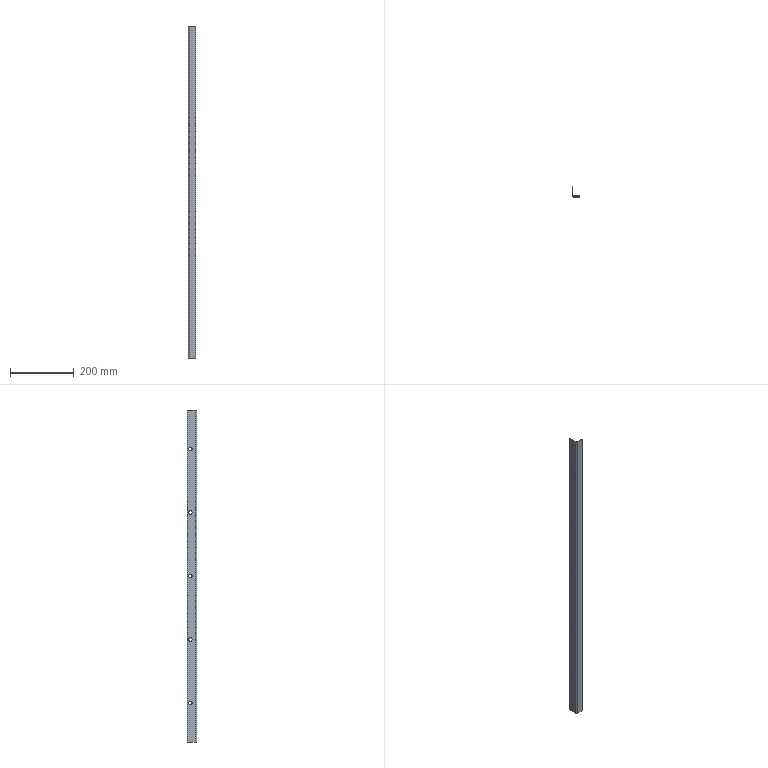Part | STEP file | 750038321 | 1 solid | 20 faces | box 25 x 30 x 1045 mm | volume 131869 mm3 | cylinder 12 | plane 8 | commonest cylinder face diameters 10.5 x10 5 x1 10 x1
STEP:
#1=CARTESIAN_POINT('',(2.5,25.25,200.));
#2=VERTEX_POINT('',#1);
#3=CARTESIAN_POINT('',(2.5,14.75,200.));
#4=VERTEX_POINT('',#3);
#5=CARTESIAN_POINT('',(2.5,20.,200.));
#6=DIRECTION('',(-1.,0.,0.));
#7=DIRECTION('',(0.,-1.,0.));
#8=AXIS2_PLACEMENT_3D('',#5,#6,#7);
#9=CIRCLE('',#8,5.25);
#10=EDGE_CURVE('',#2,#4,#9,.T.);
#11=ORIENTED_EDGE('',*,*,#10,.F.);
#12=CARTESIAN_POINT('',(0.,25.25,200.));
#13=VERTEX_POINT('',#12);
#14=CARTESIAN_POINT('',(1045.729,25.25,200.));
#15=DIRECTION('',(-1.,0.,0.));
#16=VECTOR('',#15,1000.);
#17=LINE('',#14,#16);
#18=EDGE_CURVE('',#2,#13,#17,.T.);
#19=ORIENTED_EDGE('',*,*,#18,.T.);
#20=CARTESIAN_POINT('',(0.,14.75,200.));
#21=VERTEX_POINT('',#20);
#22=CARTESIAN_POINT('',(0.,20.,200.));
#23=DIRECTION('',(1.,0.,0.));
#24=DIRECTION('',(0.,-1.,0.));
#25=AXIS2_PLACEMENT_3D('',#22,#23,#24);
#26=CIRCLE('',#25,5.25);
#27=EDGE_CURVE('',#21,#13,#26,.T.);
#28=ORIENTED_EDGE('',*,*,#27,.F.);
#29=CARTESIAN_POINT('',(1045.729,14.75,200.));
#30=DIRECTION('',(-1.,0.,0.));
#31=VECTOR('',#30,1000.);
#32=LINE('',#29,#31);
#33=EDGE_CURVE('',#4,#21,#32,.T.);
#34=ORIENTED_EDGE('',*,*,#33,.F.);
#35=EDGE_LOOP('',(#11,#19,#28,#34));
#36=FACE_OUTER_BOUND('',#35,.T.);
#37=CARTESIAN_POINT('',(1045.729,20.,200.));
#38=DIRECTION('',(-1.,0.,0.));
#39=DIRECTION('',(0.,-1.,0.));
#40=AXIS2_PLACEMENT_3D('',#37,#38,#39);
#41=CYLINDRICAL_SURFACE('',#40,5.25);
#42=ADVANCED_FACE('',(#36),#41,.F.);
#43=CARTESIAN_POINT('',(2.5,25.25,-200.));
#44=VERTEX_POINT('',#43);
#45=CARTESIAN_POINT('',(2.5,14.75,-200.));
#46=VERTEX_POINT('',#45);
#47=CARTESIAN_POINT('',(2.5,20.,-200.));
#48=DIRECTION('',(-1.,0.,0.));
#49=DIRECTION('',(0.,-1.,0.));
#50=AXIS2_PLACEMENT_3D('',#47,#48,#49);
#51=CIRCLE('',#50,5.25);
#52=EDGE_CURVE('',#44,#46,#51,.T.);
#53=ORIENTED_EDGE('',*,*,#52,.F.);
#54=CARTESIAN_POINT('',(0.,25.25,-200.));
#55=VERTEX_POINT('',#54);
#56=CARTESIAN_POINT('',(1045.729,25.25,-200.));
#57=DIRECTION('',(-1.,0.,0.));
#58=VECTOR('',#57,1000.);
#59=LINE('',#56,#58);
#60=EDGE_CURVE('',#44,#55,#59,.T.);
#61=ORIENTED_EDGE('',*,*,#60,.T.);
#62=CARTESIAN_POINT('',(0.,14.75,-200.));
#63=VERTEX_POINT('',#62);
#64=CARTESIAN_POINT('',(0.,20.,-200.));
#65=DIRECTION('',(1.,0.,0.));
#66=DIRECTION('',(0.,-1.,0.));
#67=AXIS2_PLACEMENT_3D('',#64,#65,#66);
#68=CIRCLE('',#67,5.25);
#69=EDGE_CURVE('',#63,#55,#68,.T.);
#70=ORIENTED_EDGE('',*,*,#69,.F.);
#71=CARTESIAN_POINT('',(1045.729,14.75,-200.));
#72=DIRECTION('',(-1.,0.,0.));
#73=VECTOR('',#72,1000.);
#74=LINE('',#71,#73);
#75=EDGE_CURVE('',#46,#63,#74,.T.);
#76=ORIENTED_EDGE('',*,*,#75,.F.);
#77=EDGE_LOOP('',(#53,#61,#70,#76));
#78=FACE_OUTER_BOUND('',#77,.T.);
#79=CARTESIAN_POINT('',(1045.729,20.,-200.));
#80=DIRECTION('',(-1.,0.,0.));
#81=DIRECTION('',(0.,-1.,0.));
#82=AXIS2_PLACEMENT_3D('',#79,#80,#81);
#83=CYLINDRICAL_SURFACE('',#82,5.25);
#84=ADVANCED_FACE('',(#78),#83,.F.);
#85=CARTESIAN_POINT('',(2.5,25.25,-400.));
#86=VERTEX_POINT('',#85);
#87=CARTESIAN_POINT('',(2.5,14.75,-400.));
#88=VERTEX_POINT('',#87);
#89=CARTESIAN_POINT('',(2.5,20.,-400.));
#90=DIRECTION('',(-1.,0.,0.));
#91=DIRECTION('',(0.,-1.,0.));
#92=AXIS2_PLACEMENT_3D('',#89,#90,#91);
#93=CIRCLE('',#92,5.25);
#94=EDGE_CURVE('',#86,#88,#93,.T.);
#95=ORIENTED_EDGE('',*,*,#94,.F.);
#96=CARTESIAN_POINT('',(0.,25.25,-400.));
#97=VERTEX_POINT('',#96);
#98=CARTESIAN_POINT('',(1045.729,25.25,-400.));
#99=DIRECTION('',(-1.,0.,0.));
#100=VECTOR('',#99,1000.);
#101=LINE('',#98,#100);
#102=EDGE_CURVE('',#86,#97,#101,.T.);
#103=ORIENTED_EDGE('',*,*,#102,.T.);
#104=CARTESIAN_POINT('',(0.,14.75,-400.));
#105=VERTEX_POINT('',#104);
#106=CARTESIAN_POINT('',(0.,20.,-400.));
#107=DIRECTION('',(1.,0.,0.));
#108=DIRECTION('',(0.,-1.,0.));
#109=AXIS2_PLACEMENT_3D('',#106,#107,#108);
#110=CIRCLE('',#109,5.25);
#111=EDGE_CURVE('',#105,#97,#110,.T.);
#112=ORIENTED_EDGE('',*,*,#111,.F.);
#113=CARTESIAN_POINT('',(1045.729,14.75,-400.));
#114=DIRECTION('',(-1.,0.,0.));
#115=VECTOR('',#114,1000.);
#116=LINE('',#113,#115);
#117=EDGE_CURVE('',#88,#105,#116,.T.);
#118=ORIENTED_EDGE('',*,*,#117,.F.);
#119=EDGE_LOOP('',(#95,#103,#112,#118));
#120=FACE_OUTER_BOUND('',#119,.T.);
#121=CARTESIAN_POINT('',(1045.729,20.,-400.));
#122=DIRECTION('',(-1.,0.,0.));
#123=DIRECTION('',(0.,-1.,0.));
#124=AXIS2_PLACEMENT_3D('',#121,#122,#123);
#125=CYLINDRICAL_SURFACE('',#124,5.25);
#126=ADVANCED_FACE('',(#120),#125,.F.);
#127=CARTESIAN_POINT('',(2.5,25.25,0.));
#128=VERTEX_POINT('',#127);
#129=CARTESIAN_POINT('',(2.5,14.75,0.));
#130=VERTEX_POINT('',#129);
#131=CARTESIAN_POINT('',(2.5,20.,0.));
#132=DIRECTION('',(-1.,0.,0.));
#133=DIRECTION('',(0.,-1.,0.));
#134=AXIS2_PLACEMENT_3D('',#131,#132,#133);
#135=CIRCLE('',#134,5.25);
#136=EDGE_CURVE('',#128,#130,#135,.T.);
#137=ORIENTED_EDGE('',*,*,#136,.F.);
#138=CARTESIAN_POINT('',(0.,25.25,0.));
#139=VERTEX_POINT('',#138);
#140=CARTESIAN_POINT('',(1045.729,25.25,0.));
#141=DIRECTION('',(-1.,0.,0.));
#142=VECTOR('',#141,1000.);
#143=LINE('',#140,#142);
#144=EDGE_CURVE('',#128,#139,#143,.T.);
#145=ORIENTED_EDGE('',*,*,#144,.T.);
#146=CARTESIAN_POINT('',(0.,14.75,0.));
#147=VERTEX_POINT('',#146);
#148=CARTESIAN_POINT('',(0.,20.,0.));
#149=DIRECTION('',(1.,0.,0.));
#150=DIRECTION('',(0.,-1.,0.));
#151=AXIS2_PLACEMENT_3D('',#148,#149,#150);
#152=CIRCLE('',#151,5.25);
#153=EDGE_CURVE('',#147,#139,#152,.T.);
#154=ORIENTED_EDGE('',*,*,#153,.F.);
#155=CARTESIAN_POINT('',(1045.729,14.75,0.));
#156=DIRECTION('',(-1.,0.,0.));
#157=VECTOR('',#156,1000.);
#158=LINE('',#155,#157);
#159=EDGE_CURVE('',#130,#147,#158,.T.);
#160=ORIENTED_EDGE('',*,*,#159,.F.);
#161=EDGE_LOOP('',(#137,#145,#154,#160));
#162=FACE_OUTER_BOUND('',#161,.T.);
#163=CARTESIAN_POINT('',(1045.729,20.,0.));
#164=DIRECTION('',(-1.,0.,0.));
#165=DIRECTION('',(0.,-1.,0.));
#166=AXIS2_PLACEMENT_3D('',#163,#164,#165);
#167=CYLINDRICAL_SURFACE('',#166,5.25);
#168=ADVANCED_FACE('',(#162),#167,.F.);
#169=CARTESIAN_POINT('',(2.5,25.25,400.));
#170=VERTEX_POINT('',#169);
#171=CARTESIAN_POINT('',(2.5,14.75,400.));
#172=VERTEX_POINT('',#171);
#173=CARTESIAN_POINT('',(2.5,20.,400.));
#174=DIRECTION('',(-1.,0.,0.));
#175=DIRECTION('',(0.,-1.,0.));
#176=AXIS2_PLACEMENT_3D('',#173,#174,#175);
#177=CIRCLE('',#176,5.25);
#178=EDGE_CURVE('',#170,#172,#177,.T.);
#179=ORIENTED_EDGE('',*,*,#178,.F.);
#180=CARTESIAN_POINT('',(0.,25.25,400.));
#181=VERTEX_POINT('',#180);
#182=CARTESIAN_POINT('',(1045.729,25.25,400.));
#183=DIRECTION('',(-1.,0.,0.));
#184=VECTOR('',#183,1000.);
#185=LINE('',#182,#184);
#186=EDGE_CURVE('',#170,#181,#185,.T.);
#187=ORIENTED_EDGE('',*,*,#186,.T.);
#188=CARTESIAN_POINT('',(0.,14.75,400.));
#189=VERTEX_POINT('',#188);
#190=CARTESIAN_POINT('',(0.,20.,400.));
#191=DIRECTION('',(1.,0.,0.));
#192=DIRECTION('',(0.,-1.,0.));
#193=AXIS2_PLACEMENT_3D('',#190,#191,#192);
#194=CIRCLE('',#193,5.25);
#195=EDGE_CURVE('',#189,#181,#194,.T.);
#196=ORIENTED_EDGE('',*,*,#195,.F.);
#197=CARTESIAN_POINT('',(1045.729,14.75,400.));
#198=DIRECTION('',(-1.,0.,0.));
#199=VECTOR('',#198,1000.);
#200=LINE('',#197,#199);
#201=EDGE_CURVE('',#172,#189,#200,.T.);
#202=ORIENTED_EDGE('',*,*,#201,.F.);
#203=EDGE_LOOP('',(#179,#187,#196,#202));
#204=FACE_OUTER_BOUND('',#203,.T.);
#205=CARTESIAN_POINT('',(1045.729,20.,400.));
#206=DIRECTION('',(-1.,0.,0.));
#207=DIRECTION('',(0.,-1.,0.));
#208=AXIS2_PLACEMENT_3D('',#205,#206,#207);
#209=CYLINDRICAL_SURFACE('',#208,5.25);
#210=ADVANCED_FACE('',(#204),#209,.F.);
#211=CARTESIAN_POINT('',(0.,5.,522.5));
#212=VERTEX_POINT('',#211);
#213=CARTESIAN_POINT('',(0.,30.,522.5));
#214=VERTEX_POINT('',#213);
#215=CARTESIAN_POINT('',(0.,0.,522.5));
#216=DIRECTION('',(0.,1.,0.));
#217=VECTOR('',#216,1000.);
#218=LINE('',#215,#217);
#219=EDGE_CURVE('',#212,#214,#218,.T.);
#220=ORIENTED_EDGE('',*,*,#219,.T.);
#221=CARTESIAN_POINT('',(0.,30.,-522.5));
#222=VERTEX_POINT('',#221);
#223=CARTESIAN_POINT('',(0.,30.,522.5));
#224=DIRECTION('',(0.,0.,-1.));
#225=VECTOR('',#224,1000.);
#226=LINE('',#223,#225);
#227=EDGE_CURVE('',#214,#222,#226,.T.);
#228=ORIENTED_EDGE('',*,*,#227,.T.);
#229=CARTESIAN_POINT('',(0.,5.,-522.5));
#230=VERTEX_POINT('',#229);
#231=CARTESIAN_POINT('',(0.,0.,-522.5));
#232=DIRECTION('',(0.,-1.,0.));
#233=VECTOR('',#232,1000.);
#234=LINE('',#231,#233);
#235=EDGE_CURVE('',#222,#230,#234,.T.);
#236=ORIENTED_EDGE('',*,*,#235,.T.);
#237=CARTESIAN_POINT('',(0.,5.,522.5));
#238=DIRECTION('',(0.,0.,1.));
#239=VECTOR('',#238,1000.);
#240=LINE('',#237,#239);
#241=EDGE_CURVE('',#230,#212,#240,.T.);
#242=ORIENTED_EDGE('',*,*,#241,.T.);
#243=EDGE_LOOP('',(#220,#228,#236,#242));
#244=FACE_OUTER_BOUND('',#243,.T.);
#245=ORIENTED_EDGE('',*,*,#27,.T.);
#246=CARTESIAN_POINT('',(0.,20.,200.));
#247=DIRECTION('',(1.,0.,0.));
#248=DIRECTION('',(0.,-1.,0.));
#249=AXIS2_PLACEMENT_3D('',#246,#247,#248);
#250=CIRCLE('',#249,5.25);
#251=EDGE_CURVE('',#13,#21,#250,.T.);
#252=ORIENTED_EDGE('',*,*,#251,.T.);
#253=EDGE_LOOP('',(#245,#252));
#254=FACE_BOUND('',#253,.T.);
#255=ORIENTED_EDGE('',*,*,#69,.T.);
#256=CARTESIAN_POINT('',(0.,20.,-200.));
#257=DIRECTION('',(1.,0.,0.));
#258=DIRECTION('',(0.,-1.,0.));
#259=AXIS2_PLACEMENT_3D('',#256,#257,#258);
#260=CIRCLE('',#259,5.25);
#261=EDGE_CURVE('',#55,#63,#260,.T.);
#262=ORIENTED_EDGE('',*,*,#261,.T.);
#263=EDGE_LOOP('',(#255,#262));
#264=FACE_BOUND('',#263,.T.);
#265=ORIENTED_EDGE('',*,*,#111,.T.);
#266=CARTESIAN_POINT('',(0.,20.,-400.));
#267=DIRECTION('',(1.,0.,0.));
#268=DIRECTION('',(0.,-1.,0.));
#269=AXIS2_PLACEMENT_3D('',#266,#267,#268);
#270=CIRCLE('',#269,5.25);
#271=EDGE_CURVE('',#97,#105,#270,.T.);
#272=ORIENTED_EDGE('',*,*,#271,.T.);
#273=EDGE_LOOP('',(#265,#272));
#274=FACE_BOUND('',#273,.T.);
#275=ORIENTED_EDGE('',*,*,#153,.T.);
#276=CARTESIAN_POINT('',(0.,20.,0.));
#277=DIRECTION('',(1.,0.,0.));
#278=DIRECTION('',(0.,-1.,0.));
#279=AXIS2_PLACEMENT_3D('',#276,#277,#278);
#280=CIRCLE('',#279,5.25);
#281=EDGE_CURVE('',#139,#147,#280,.T.);
#282=ORIENTED_EDGE('',*,*,#281,.T.);
#283=EDGE_LOOP('',(#275,#282));
#284=FACE_BOUND('',#283,.T.);
#285=ORIENTED_EDGE('',*,*,#195,.T.);
#286=CARTESIAN_POINT('',(0.,20.,400.));
#287=DIRECTION('',(1.,0.,0.));
#288=DIRECTION('',(0.,-1.,0.));
#289=AXIS2_PLACEMENT_3D('',#286,#287,#288);
#290=CIRCLE('',#289,5.25);
#291=EDGE_CURVE('',#181,#189,#290,.T.);
#292=ORIENTED_EDGE('',*,*,#291,.T.);
#293=EDGE_LOOP('',(#285,#292));
#294=FACE_BOUND('',#293,.T.);
#295=CARTESIAN_POINT('',(0.,0.,522.5));
#296=DIRECTION('',(-1.,0.,0.));
#297=DIRECTION('',(0.,-1.,0.));
#298=AXIS2_PLACEMENT_3D('',#295,#296,#297);
#299=PLANE('',#298);
#300=ADVANCED_FACE('',(#244,#254,#264,#274,#284,#294),#299,.T.);
#301=CARTESIAN_POINT('',(2.5,30.,-522.5));
#302=VERTEX_POINT('',#301);
#303=CARTESIAN_POINT('',(0.,30.,-522.5));
#304=DIRECTION('',(-1.,0.,0.));
#305=VECTOR('',#304,1000.);
#306=LINE('',#303,#305);
#307=EDGE_CURVE('',#302,#222,#306,.T.);
#308=ORIENTED_EDGE('',*,*,#307,.T.);
#309=ORIENTED_EDGE('',*,*,#227,.F.);
#310=CARTESIAN_POINT('',(2.5,30.,522.5));
#311=VERTEX_POINT('',#310);
#312=CARTESIAN_POINT('',(0.,30.,522.5));
#313=DIRECTION('',(1.,0.,0.));
#314=VECTOR('',#313,1000.);
#315=LINE('',#312,#314);
#316=EDGE_CURVE('',#214,#311,#315,.T.);
#317=ORIENTED_EDGE('',*,*,#316,.T.);
#318=CARTESIAN_POINT('',(2.5,30.,522.5));
#319=DIRECTION('',(0.,0.,-1.));
#320=VECTOR('',#319,1000.);
#321=LINE('',#318,#320);
#322=EDGE_CURVE('',#311,#302,#321,.T.);
#323=ORIENTED_EDGE('',*,*,#322,.T.);
#324=EDGE_LOOP('',(#308,#309,#317,#323));
#325=FACE_OUTER_BOUND('',#324,.T.);
#326=CARTESIAN_POINT('',(0.,30.,522.5));
#327=DIRECTION('',(0.,1.,0.));
#328=DIRECTION('',(-1.,0.,0.));
#329=AXIS2_PLACEMENT_3D('',#326,#327,#328);
#330=PLANE('',#329);
#331=ADVANCED_FACE('',(#325),#330,.T.);
#332=CARTESIAN_POINT('',(2.5,5.,522.5));
#333=VERTEX_POINT('',#332);
#334=CARTESIAN_POINT('',(2.5,0.,522.5));
#335=DIRECTION('',(0.,1.,0.));
#336=VECTOR('',#335,1000.);
#337=LINE('',#334,#336);
#338=EDGE_CURVE('',#333,#311,#337,.T.);
#339=ORIENTED_EDGE('',*,*,#338,.T.);
#340=ORIENTED_EDGE('',*,*,#316,.F.);
#341=ORIENTED_EDGE('',*,*,#219,.F.);
#342=CARTESIAN_POINT('',(5.,0.,522.5));
#343=VERTEX_POINT('',#342);
#344=CARTESIAN_POINT('',(5.,5.,522.5));
#345=DIRECTION('',(0.,0.,1.));
#346=DIRECTION('',(-1.,0.,0.));
#347=AXIS2_PLACEMENT_3D('',#344,#345,#346);
#348=CIRCLE('',#347,5.);
#349=EDGE_CURVE('',#212,#343,#348,.T.);
#350=ORIENTED_EDGE('',*,*,#349,.T.);
#351=CARTESIAN_POINT('',(25.,0.,522.5));
#352=VERTEX_POINT('',#351);
#353=CARTESIAN_POINT('',(0.,0.,522.5));
#354=DIRECTION('',(1.,0.,0.));
#355=VECTOR('',#354,1000.);
#356=LINE('',#353,#355);
#357=EDGE_CURVE('',#343,#352,#356,.T.);
#358=ORIENTED_EDGE('',*,*,#357,.T.);
#359=CARTESIAN_POINT('',(25.,2.5,522.5));
#360=VERTEX_POINT('',#359);
#361=CARTESIAN_POINT('',(25.,0.,522.5));
#362=DIRECTION('',(0.,1.,0.));
#363=VECTOR('',#362,1000.);
#364=LINE('',#361,#363);
#365=EDGE_CURVE('',#352,#360,#364,.T.);
#366=ORIENTED_EDGE('',*,*,#365,.T.);
#367=CARTESIAN_POINT('',(5.,2.5,522.5));
#368=VERTEX_POINT('',#367);
#369=CARTESIAN_POINT('',(0.,2.5,522.5));
#370=DIRECTION('',(-1.,0.,0.));
#371=VECTOR('',#370,1000.);
#372=LINE('',#369,#371);
#373=EDGE_CURVE('',#360,#368,#372,.T.);
#374=ORIENTED_EDGE('',*,*,#373,.T.);
#375=CARTESIAN_POINT('',(5.,5.,522.5));
#376=DIRECTION('',(0.,0.,-1.));
#377=DIRECTION('',(-1.,0.,0.));
#378=AXIS2_PLACEMENT_3D('',#375,#376,#377);
#379=CIRCLE('',#378,2.5);
#380=EDGE_CURVE('',#368,#333,#379,.T.);
#381=ORIENTED_EDGE('',*,*,#380,.T.);
#382=EDGE_LOOP('',(#339,#340,#341,#350,#358,#366,#374,#381));
#383=FACE_OUTER_BOUND('',#382,.T.);
#384=CARTESIAN_POINT('',(0.,0.,522.5));
#385=DIRECTION('',(0.,0.,1.));
#386=DIRECTION('',(1.,0.,0.));
#387=AXIS2_PLACEMENT_3D('',#384,#385,#386);
#388=PLANE('',#387);
#389=ADVANCED_FACE('',(#383),#388,.T.);
#390=ORIENTED_EDGE('',*,*,#349,.F.);
#391=ORIENTED_EDGE('',*,*,#241,.F.);
#392=CARTESIAN_POINT('',(5.,0.,-522.5));
#393=VERTEX_POINT('',#392);
#394=CARTESIAN_POINT('',(5.,5.,-522.5));
#395=DIRECTION('',(0.,0.,1.));
#396=DIRECTION('',(-1.,0.,0.));
#397=AXIS2_PLACEMENT_3D('',#394,#395,#396);
#398=CIRCLE('',#397,5.);
#399=EDGE_CURVE('',#230,#393,#398,.T.);
#400=ORIENTED_EDGE('',*,*,#399,.T.);
#401=CARTESIAN_POINT('',(5.,0.,522.5));
#402=DIRECTION('',(0.,0.,1.));
#403=VECTOR('',#402,1000.);
#404=LINE('',#401,#403);
#405=EDGE_CURVE('',#393,#343,#404,.T.);
#406=ORIENTED_EDGE('',*,*,#405,.T.);
#407=EDGE_LOOP('',(#390,#391,#400,#406));
#408=FACE_OUTER_BOUND('',#407,.T.);
#409=CARTESIAN_POINT('',(5.,5.,522.5));
#410=DIRECTION('',(0.,0.,-1.));
#411=DIRECTION('',(-1.,0.,0.));
#412=AXIS2_PLACEMENT_3D('',#409,#410,#411);
#413=CYLINDRICAL_SURFACE('',#412,5.);
#414=ADVANCED_FACE('',(#408),#413,.T.);
#415=ORIENTED_EDGE('',*,*,#399,.F.);
#416=ORIENTED_EDGE('',*,*,#235,.F.);
#417=ORIENTED_EDGE('',*,*,#307,.F.);
#418=CARTESIAN_POINT('',(2.5,5.,-522.5));
#419=VERTEX_POINT('',#418);
#420=CARTESIAN_POINT('',(2.5,0.,-522.5));
#421=DIRECTION('',(0.,1.,0.));
#422=VECTOR('',#421,1000.);
#423=LINE('',#420,#422);
#424=EDGE_CURVE('',#419,#302,#423,.T.);
#425=ORIENTED_EDGE('',*,*,#424,.F.);
#426=CARTESIAN_POINT('',(5.,2.5,-522.5));
#427=VERTEX_POINT('',#426);
#428=CARTESIAN_POINT('',(5.,5.,-522.5));
#429=DIRECTION('',(0.,0.,-1.));
#430=DIRECTION('',(-1.,0.,0.));
#431=AXIS2_PLACEMENT_3D('',#428,#429,#430);
#432=CIRCLE('',#431,2.5);
#433=EDGE_CURVE('',#427,#419,#432,.T.);
#434=ORIENTED_EDGE('',*,*,#433,.F.);
#435=CARTESIAN_POINT('',(25.,2.5,-522.5));
#436=VERTEX_POINT('',#435);
#437=CARTESIAN_POINT('',(25.,2.5,-522.5));
#438=DIRECTION('',(-1.,0.,0.));
#439=VECTOR('',#438,1000.);
#440=LINE('',#437,#439);
#441=EDGE_CURVE('',#436,#427,#440,.T.);
#442=ORIENTED_EDGE('',*,*,#441,.F.);
#443=CARTESIAN_POINT('',(25.,0.,-522.5));
#444=VERTEX_POINT('',#443);
#445=CARTESIAN_POINT('',(25.,0.,-522.5));
#446=DIRECTION('',(0.,1.,0.));
#447=VECTOR('',#446,1000.);
#448=LINE('',#445,#447);
#449=EDGE_CURVE('',#444,#436,#448,.T.);
#450=ORIENTED_EDGE('',*,*,#449,.F.);
#451=CARTESIAN_POINT('',(25.,0.,-522.5));
#452=DIRECTION('',(1.,0.,0.));
#453=VECTOR('',#452,1000.);
#454=LINE('',#451,#453);
#455=EDGE_CURVE('',#393,#444,#454,.T.);
#456=ORIENTED_EDGE('',*,*,#455,.F.);
#457=EDGE_LOOP('',(#415,#416,#417,#425,#434,#442,#450,#456));
#458=FACE_OUTER_BOUND('',#457,.T.);
#459=CARTESIAN_POINT('',(25.,0.,-522.5));
#460=DIRECTION('',(0.,0.,1.));
#461=DIRECTION('',(1.,0.,0.));
#462=AXIS2_PLACEMENT_3D('',#459,#460,#461);
#463=PLANE('',#462);
#464=ADVANCED_FACE('',(#458),#463,.F.);
#465=ORIENTED_EDGE('',*,*,#18,.F.);
#466=CARTESIAN_POINT('',(2.5,20.,200.));
#467=DIRECTION('',(-1.,0.,0.));
#468=DIRECTION('',(0.,-1.,0.));
#469=AXIS2_PLACEMENT_3D('',#466,#467,#468);
#470=CIRCLE('',#469,5.25);
#471=EDGE_CURVE('',#4,#2,#470,.T.);
#472=ORIENTED_EDGE('',*,*,#471,.F.);
#473=ORIENTED_EDGE('',*,*,#33,.T.);
#474=ORIENTED_EDGE('',*,*,#251,.F.);
#475=EDGE_LOOP('',(#465,#472,#473,#474));
#476=FACE_OUTER_BOUND('',#475,.T.);
#477=CARTESIAN_POINT('',(1045.729,20.,200.));
#478=DIRECTION('',(-1.,0.,0.));
#479=DIRECTION('',(0.,-1.,0.));
#480=AXIS2_PLACEMENT_3D('',#477,#478,#479);
#481=CYLINDRICAL_SURFACE('',#480,5.25);
#482=ADVANCED_FACE('',(#476),#481,.F.);
#483=ORIENTED_EDGE('',*,*,#60,.F.);
#484=CARTESIAN_POINT('',(2.5,20.,-200.));
#485=DIRECTION('',(-1.,0.,0.));
#486=DIRECTION('',(0.,-1.,0.));
#487=AXIS2_PLACEMENT_3D('',#484,#485,#486);
#488=CIRCLE('',#487,5.25);
#489=EDGE_CURVE('',#46,#44,#488,.T.);
#490=ORIENTED_EDGE('',*,*,#489,.F.);
#491=ORIENTED_EDGE('',*,*,#75,.T.);
#492=ORIENTED_EDGE('',*,*,#261,.F.);
#493=EDGE_LOOP('',(#483,#490,#491,#492));
#494=FACE_OUTER_BOUND('',#493,.T.);
#495=CARTESIAN_POINT('',(1045.729,20.,-200.));
#496=DIRECTION('',(-1.,0.,0.));
#497=DIRECTION('',(0.,-1.,0.));
#498=AXIS2_PLACEMENT_3D('',#495,#496,#497);
#499=CYLINDRICAL_SURFACE('',#498,5.25);
#500=ADVANCED_FACE('',(#494),#499,.F.);
#501=ORIENTED_EDGE('',*,*,#102,.F.);
#502=CARTESIAN_POINT('',(2.5,20.,-400.));
#503=DIRECTION('',(-1.,0.,0.));
#504=DIRECTION('',(0.,-1.,0.));
#505=AXIS2_PLACEMENT_3D('',#502,#503,#504);
#506=CIRCLE('',#505,5.25);
#507=EDGE_CURVE('',#88,#86,#506,.T.);
#508=ORIENTED_EDGE('',*,*,#507,.F.);
#509=ORIENTED_EDGE('',*,*,#117,.T.);
#510=ORIENTED_EDGE('',*,*,#271,.F.);
#511=EDGE_LOOP('',(#501,#508,#509,#510));
#512=FACE_OUTER_BOUND('',#511,.T.);
#513=CARTESIAN_POINT('',(1045.729,20.,-400.));
#514=DIRECTION('',(-1.,0.,0.));
#515=DIRECTION('',(0.,-1.,0.));
#516=AXIS2_PLACEMENT_3D('',#513,#514,#515);
#517=CYLINDRICAL_SURFACE('',#516,5.25);
#518=ADVANCED_FACE('',(#512),#517,.F.);
#519=ORIENTED_EDGE('',*,*,#144,.F.);
#520=CARTESIAN_POINT('',(2.5,20.,0.));
#521=DIRECTION('',(-1.,0.,0.));
#522=DIRECTION('',(0.,-1.,0.));
#523=AXIS2_PLACEMENT_3D('',#520,#521,#522);
#524=CIRCLE('',#523,5.25);
#525=EDGE_CURVE('',#130,#128,#524,.T.);
#526=ORIENTED_EDGE('',*,*,#525,.F.);
#527=ORIENTED_EDGE('',*,*,#159,.T.);
#528=ORIENTED_EDGE('',*,*,#281,.F.);
#529=EDGE_LOOP('',(#519,#526,#527,#528));
#530=FACE_OUTER_BOUND('',#529,.T.);
#531=CARTESIAN_POINT('',(1045.729,20.,0.));
#532=DIRECTION('',(-1.,0.,0.));
#533=DIRECTION('',(0.,-1.,0.));
#534=AXIS2_PLACEMENT_3D('',#531,#532,#533);
#535=CYLINDRICAL_SURFACE('',#534,5.25);
#536=ADVANCED_FACE('',(#530),#535,.F.);
#537=ORIENTED_EDGE('',*,*,#186,.F.);
#538=CARTESIAN_POINT('',(2.5,20.,400.));
#539=DIRECTION('',(-1.,0.,0.));
#540=DIRECTION('',(0.,-1.,0.));
#541=AXIS2_PLACEMENT_3D('',#538,#539,#540);
#542=CIRCLE('',#541,5.25);
#543=EDGE_CURVE('',#172,#170,#542,.T.);
#544=ORIENTED_EDGE('',*,*,#543,.F.);
#545=ORIENTED_EDGE('',*,*,#201,.T.);
#546=ORIENTED_EDGE('',*,*,#291,.F.);
#547=EDGE_LOOP('',(#537,#544,#545,#546));
#548=FACE_OUTER_BOUND('',#547,.T.);
#549=CARTESIAN_POINT('',(1045.729,20.,400.));
#550=DIRECTION('',(-1.,0.,0.));
#551=DIRECTION('',(0.,-1.,0.));
#552=AXIS2_PLACEMENT_3D('',#549,#550,#551);
#553=CYLINDRICAL_SURFACE('',#552,5.25);
#554=ADVANCED_FACE('',(#548),#553,.F.);
#555=ORIENTED_EDGE('',*,*,#322,.F.);
#556=ORIENTED_EDGE('',*,*,#338,.F.);
#557=CARTESIAN_POINT('',(2.5,5.,522.5));
#558=DIRECTION('',(0.,0.,1.));
#559=VECTOR('',#558,1000.);
#560=LINE('',#557,#559);
#561=EDGE_CURVE('',#419,#333,#560,.T.);
#562=ORIENTED_EDGE('',*,*,#561,.F.);
#563=ORIENTED_EDGE('',*,*,#424,.T.);
#564=EDGE_LOOP('',(#555,#556,#562,#563));
#565=FACE_OUTER_BOUND('',#564,.T.);
#566=ORIENTED_EDGE('',*,*,#471,.T.);
#567=ORIENTED_EDGE('',*,*,#10,.T.);
#568=EDGE_LOOP('',(#566,#567));
#569=FACE_BOUND('',#568,.T.);
#570=ORIENTED_EDGE('',*,*,#489,.T.);
#571=ORIENTED_EDGE('',*,*,#52,.T.);
#572=EDGE_LOOP('',(#570,#571));
#573=FACE_BOUND('',#572,.T.);
#574=ORIENTED_EDGE('',*,*,#507,.T.);
#575=ORIENTED_EDGE('',*,*,#94,.T.);
#576=EDGE_LOOP('',(#574,#575));
#577=FACE_BOUND('',#576,.T.);
#578=ORIENTED_EDGE('',*,*,#525,.T.);
#579=ORIENTED_EDGE('',*,*,#136,.T.);
#580=EDGE_LOOP('',(#578,#579));
#581=FACE_BOUND('',#580,.T.);
#582=ORIENTED_EDGE('',*,*,#543,.T.);
#583=ORIENTED_EDGE('',*,*,#178,.T.);
#584=EDGE_LOOP('',(#582,#583));
#585=FACE_BOUND('',#584,.T.);
#586=CARTESIAN_POINT('',(2.5,0.,522.5));
#587=DIRECTION('',(-1.,0.,0.));
#588=DIRECTION('',(0.,-1.,0.));
#589=AXIS2_PLACEMENT_3D('',#586,#587,#588);
#590=PLANE('',#589);
#591=ADVANCED_FACE('',(#565,#569,#573,#577,#581,#585),#590,.F.);
#592=ORIENTED_EDGE('',*,*,#561,.T.);
#593=ORIENTED_EDGE('',*,*,#380,.F.);
#594=CARTESIAN_POINT('',(5.,2.5,522.5));
#595=DIRECTION('',(0.,0.,1.));
#596=VECTOR('',#595,1000.);
#597=LINE('',#594,#596);
#598=EDGE_CURVE('',#427,#368,#597,.T.);
#599=ORIENTED_EDGE('',*,*,#598,.F.);
#600=ORIENTED_EDGE('',*,*,#433,.T.);
#601=EDGE_LOOP('',(#592,#593,#599,#600));
#602=FACE_OUTER_BOUND('',#601,.T.);
#603=CARTESIAN_POINT('',(5.,5.,522.5));
#604=DIRECTION('',(0.,0.,-1.));
#605=DIRECTION('',(-1.,0.,0.));
#606=AXIS2_PLACEMENT_3D('',#603,#604,#605);
#607=CYLINDRICAL_SURFACE('',#606,2.5);
#608=ADVANCED_FACE('',(#602),#607,.F.);
#609=ORIENTED_EDGE('',*,*,#598,.T.);
#610=ORIENTED_EDGE('',*,*,#373,.F.);
#611=CARTESIAN_POINT('',(25.,2.5,522.5));
#612=DIRECTION('',(0.,0.,1.));
#613=VECTOR('',#612,1000.);
#614=LINE('',#611,#613);
#615=EDGE_CURVE('',#436,#360,#614,.T.);
#616=ORIENTED_EDGE('',*,*,#615,.F.);
#617=ORIENTED_EDGE('',*,*,#441,.T.);
#618=EDGE_LOOP('',(#609,#610,#616,#617));
#619=FACE_OUTER_BOUND('',#618,.T.);
#620=CARTESIAN_POINT('',(25.,2.5,522.5));
#621=DIRECTION('',(0.,-1.,0.));
#622=DIRECTION('',(0.,0.,-1.));
#623=AXIS2_PLACEMENT_3D('',#620,#621,#622);
#624=PLANE('',#623);
#625=ADVANCED_FACE('',(#619),#624,.F.);
#626=ORIENTED_EDGE('',*,*,#365,.F.);
#627=CARTESIAN_POINT('',(25.,0.,522.5));
#628=DIRECTION('',(0.,0.,1.));
#629=VECTOR('',#628,1000.);
#630=LINE('',#627,#629);
#631=EDGE_CURVE('',#444,#352,#630,.T.);
#632=ORIENTED_EDGE('',*,*,#631,.F.);
#633=ORIENTED_EDGE('',*,*,#449,.T.);
#634=ORIENTED_EDGE('',*,*,#615,.T.);
#635=EDGE_LOOP('',(#626,#632,#633,#634));
#636=FACE_OUTER_BOUND('',#635,.T.);
#637=CARTESIAN_POINT('',(25.,0.,522.5));
#638=DIRECTION('',(-1.,0.,0.));
#639=DIRECTION('',(0.,0.,1.));
#640=AXIS2_PLACEMENT_3D('',#637,#638,#639);
#641=PLANE('',#640);
#642=ADVANCED_FACE('',(#636),#641,.F.);
#643=ORIENTED_EDGE('',*,*,#357,.F.);
#644=ORIENTED_EDGE('',*,*,#405,.F.);
#645=ORIENTED_EDGE('',*,*,#455,.T.);
#646=ORIENTED_EDGE('',*,*,#631,.T.);
#647=EDGE_LOOP('',(#643,#644,#645,#646));
#648=FACE_OUTER_BOUND('',#647,.T.);
#649=CARTESIAN_POINT('',(25.,0.,522.5));
#650=DIRECTION('',(0.,-1.,0.));
#651=DIRECTION('',(0.,0.,-1.));
#652=AXIS2_PLACEMENT_3D('',#649,#650,#651);
#653=PLANE('',#652);
#654=ADVANCED_FACE('',(#648),#653,.T.);
#655=CLOSED_SHELL('',(#42,#84,#126,#168,#210,#300,#331,#389,#414,#464,#482,#500,#518,#536,#554,#591,#608,#625,#642,#654));
#656=MANIFOLD_SOLID_BREP('',#655);
#657=CARTESIAN_POINT('',(0.,0.,0.));
#658=DIRECTION('',(0.,0.,1.));
#659=DIRECTION('',(1.,0.,0.));
#660=AXIS2_PLACEMENT_3D('',#657,#658,#659);
#661=(LENGTH_UNIT()NAMED_UNIT(*)SI_UNIT(.MILLI.,.METRE.));
#662=UNCERTAINTY_MEASURE_WITH_UNIT(LENGTH_MEASURE(0.00001),#661,'','');
#663=(NAMED_UNIT(*)PLANE_ANGLE_UNIT()SI_UNIT($,.RADIAN.));
#664=(NAMED_UNIT(*)SI_UNIT($,.STERADIAN.)SOLID_ANGLE_UNIT());
#665=(GEOMETRIC_REPRESENTATION_CONTEXT(3)GLOBAL_UNCERTAINTY_ASSIGNED_CONTEXT((#662))GLOBAL_UNIT_ASSIGNED_CONTEXT((#661,#663,#664))REPRESENTATION_CONTEXT('',''));
#666=ADVANCED_BREP_SHAPE_REPRESENTATION('',(#656,#660),#665);